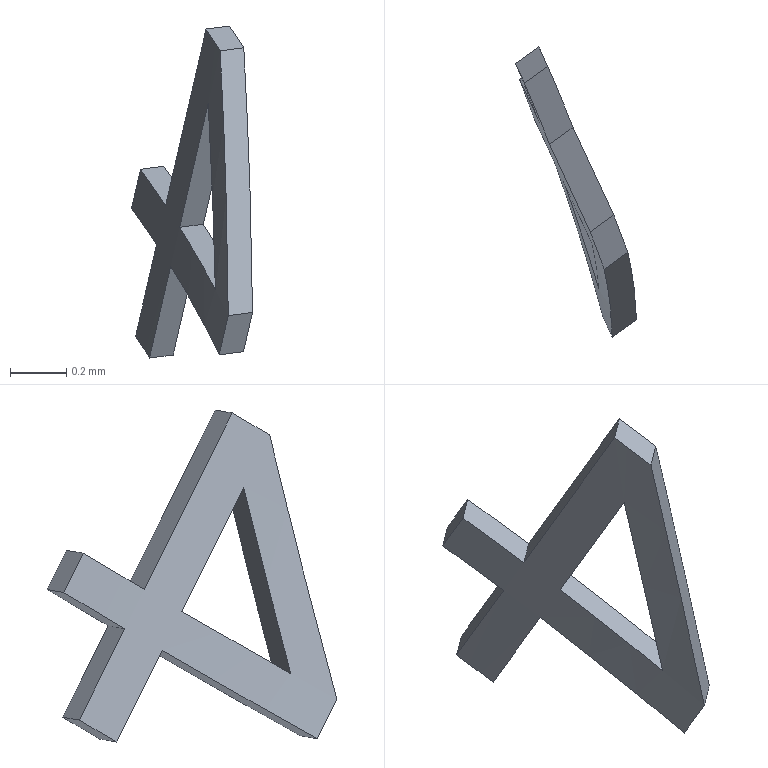Part | SolidWorks | features BaseBody 1 | 1 solid | 16 faces | box 0.4319 x 1.035 x 1.185 mm | volume 0.04699 mm3 | plane 14 | cylinder 2 | commonest cylinder face diameters 16.8 x1 17 x1
STEP:
#1=CARTESIAN_POINT('',(1974.754,-241.68,993.534));
#2=VERTEX_POINT('',#1);
#3=CARTESIAN_POINT('',(1974.725,-241.439,994.479));
#4=VERTEX_POINT('',#3);
#5=CARTESIAN_POINT('',(1974.754,-241.68,993.534));
#6=CARTESIAN_POINT('',(1974.752,-241.595,993.848));
#7=CARTESIAN_POINT('',(1974.742,-241.515,994.163));
#8=CARTESIAN_POINT('',(1974.725,-241.439,994.479));
#9=B_SPLINE_CURVE_WITH_KNOTS('',3,(#5,#6,#7,#8),.UNSPECIFIED.,.F.,.F.,(4,4),(0.,1.),.UNSPECIFIED.);
#10=EDGE_CURVE('',#2,#4,#9,.T.);
#11=ORIENTED_EDGE('',*,*,#10,.T.);
#12=CARTESIAN_POINT('',(1974.675,-241.306,994.556));
#13=VERTEX_POINT('',#12);
#14=CARTESIAN_POINT('',(1966.892,-244.458,994.777));
#15=DIRECTION('',(0.2015,-0.436,0.8771));
#16=DIRECTION('',(-0.7309,-0.6631,-0.1618));
#17=AXIS2_PLACEMENT_3D('',#14,#15,#16);
#18=CIRCLE('',#17,8.4);
#19=EDGE_CURVE('',#4,#13,#18,.T.);
#20=ORIENTED_EDGE('',*,*,#19,.T.);
#21=CARTESIAN_POINT('',(1974.53,-240.993,993.927));
#22=VERTEX_POINT('',#21);
#23=CARTESIAN_POINT('',(1975.233,-242.514,996.986));
#24=DIRECTION('',(-0.2015,0.436,-0.8771));
#25=VECTOR('',#24,1000.);
#26=LINE('',#23,#25);
#27=EDGE_CURVE('',#13,#22,#26,.T.);
#28=ORIENTED_EDGE('',*,*,#27,.T.);
#29=CARTESIAN_POINT('',(1974.441,-240.774,994.056));
#30=VERTEX_POINT('',#29);
#31=CARTESIAN_POINT('',(1966.747,-244.145,994.147));
#32=DIRECTION('',(0.2015,-0.436,0.8771));
#33=DIRECTION('',(-0.7309,-0.6631,-0.1618));
#34=AXIS2_PLACEMENT_3D('',#31,#32,#33);
#35=CIRCLE('',#34,8.4);
#36=EDGE_CURVE('',#22,#30,#35,.T.);
#37=ORIENTED_EDGE('',*,*,#36,.T.);
#38=CARTESIAN_POINT('',(1974.409,-240.705,993.916));
#39=VERTEX_POINT('',#38);
#40=CARTESIAN_POINT('',(1975.143,-242.295,997.115));
#41=DIRECTION('',(-0.2015,0.436,-0.8771));
#42=VECTOR('',#41,1000.);
#43=LINE('',#40,#42);
#44=EDGE_CURVE('',#30,#39,#43,.T.);
#45=ORIENTED_EDGE('',*,*,#44,.T.);
#46=CARTESIAN_POINT('',(1974.498,-240.923,993.787));
#47=VERTEX_POINT('',#46);
#48=CARTESIAN_POINT('',(1966.715,-244.076,994.007));
#49=DIRECTION('',(-0.2015,0.436,-0.8771));
#50=DIRECTION('',(-0.7309,-0.6631,-0.1618));
#51=AXIS2_PLACEMENT_3D('',#48,#49,#50);
#52=CIRCLE('',#51,8.4);
#53=EDGE_CURVE('',#39,#47,#52,.T.);
#54=ORIENTED_EDGE('',*,*,#53,.T.);
#55=CARTESIAN_POINT('',(1974.423,-240.761,993.46));
#56=VERTEX_POINT('',#55);
#57=CARTESIAN_POINT('',(1975.233,-242.514,996.986));
#58=DIRECTION('',(-0.2015,0.436,-0.8771));
#59=VECTOR('',#58,1000.);
#60=LINE('',#57,#59);
#61=EDGE_CURVE('',#47,#56,#60,.T.);
#62=ORIENTED_EDGE('',*,*,#61,.T.);
#63=CARTESIAN_POINT('',(1974.473,-240.894,993.382));
#64=VERTEX_POINT('',#63);
#65=CARTESIAN_POINT('',(1966.64,-243.913,993.681));
#66=DIRECTION('',(-0.2015,0.436,-0.8771));
#67=DIRECTION('',(-0.7309,-0.6631,-0.1618));
#68=AXIS2_PLACEMENT_3D('',#65,#66,#67);
#69=CIRCLE('',#68,8.4);
#70=EDGE_CURVE('',#56,#64,#69,.T.);
#71=ORIENTED_EDGE('',*,*,#70,.T.);
#72=CARTESIAN_POINT('',(1974.548,-241.057,993.709));
#73=VERTEX_POINT('',#72);
#74=CARTESIAN_POINT('',(1975.283,-242.647,996.908));
#75=DIRECTION('',(0.2015,-0.436,0.8771));
#76=VECTOR('',#75,1000.);
#77=LINE('',#74,#76);
#78=EDGE_CURVE('',#64,#73,#77,.T.);
#79=ORIENTED_EDGE('',*,*,#78,.T.);
#80=CARTESIAN_POINT('',(1974.722,-241.61,993.394));
#81=VERTEX_POINT('',#80);
#82=CARTESIAN_POINT('',(1966.715,-244.076,994.007));
#83=DIRECTION('',(-0.2015,0.436,-0.8771));
#84=DIRECTION('',(-0.7309,-0.6631,-0.1618));
#85=AXIS2_PLACEMENT_3D('',#82,#83,#84);
#86=CIRCLE('',#85,8.4);
#87=EDGE_CURVE('',#73,#81,#86,.T.);
#88=ORIENTED_EDGE('',*,*,#87,.T.);
#89=CARTESIAN_POINT('',(1975.457,-243.201,996.593));
#90=DIRECTION('',(-0.2015,0.436,-0.8771));
#91=VECTOR('',#90,1000.);
#92=LINE('',#89,#91);
#93=EDGE_CURVE('',#2,#81,#92,.T.);
#94=ORIENTED_EDGE('',*,*,#93,.F.);
#95=EDGE_LOOP('',(#11,#20,#28,#37,#45,#54,#62,#71,#79,#88,#94));
#96=FACE_OUTER_BOUND('',#95,.T.);
#97=CARTESIAN_POINT('',(1974.58,-241.126,993.849));
#98=VERTEX_POINT('',#97);
#99=CARTESIAN_POINT('',(1974.682,-241.347,994.292));
#100=VERTEX_POINT('',#99);
#101=CARTESIAN_POINT('',(1975.283,-242.647,996.908));
#102=DIRECTION('',(0.2015,-0.436,0.8771));
#103=VECTOR('',#102,1000.);
#104=LINE('',#101,#103);
#105=EDGE_CURVE('',#98,#100,#104,.T.);
#106=ORIENTED_EDGE('',*,*,#105,.T.);
#107=CARTESIAN_POINT('',(1974.708,-241.515,993.626));
#108=VERTEX_POINT('',#107);
#109=CARTESIAN_POINT('',(1974.708,-241.515,993.626));
#110=CARTESIAN_POINT('',(1974.703,-241.457,993.848));
#111=CARTESIAN_POINT('',(1974.694,-241.4,994.07));
#112=CARTESIAN_POINT('',(1974.682,-241.347,994.292));
#113=B_SPLINE_CURVE_WITH_KNOTS('',3,(#109,#110,#111,#112),.UNSPECIFIED.,.F.,.F.,(4,4),(0.,1.),.UNSPECIFIED.);
#114=EDGE_CURVE('',#108,#100,#113,.T.);
#115=ORIENTED_EDGE('',*,*,#114,.F.);
#116=CARTESIAN_POINT('',(1966.747,-244.145,994.147));
#117=DIRECTION('',(0.2015,-0.436,0.8771));
#118=DIRECTION('',(-0.7309,-0.6631,-0.1618));
#119=AXIS2_PLACEMENT_3D('',#116,#117,#118);
#120=CIRCLE('',#119,8.4);
#121=EDGE_CURVE('',#108,#98,#120,.T.);
#122=ORIENTED_EDGE('',*,*,#121,.T.);
#123=EDGE_LOOP('',(#106,#115,#122));
#124=FACE_BOUND('',#123,.T.);
#125=CARTESIAN_POINT('',(1967.45,-245.666,997.207));
#126=DIRECTION('',(0.2015,-0.436,0.8771));
#127=DIRECTION('',(-0.7309,-0.6631,-0.1618));
#128=AXIS2_PLACEMENT_3D('',#125,#126,#127);
#129=CYLINDRICAL_SURFACE('',#128,8.4);
#130=ADVANCED_FACE('',(#96,#124),#129,.F.);
#131=CARTESIAN_POINT('',(1974.84,-241.618,993.545));
#132=VERTEX_POINT('',#131);
#133=CARTESIAN_POINT('',(1974.808,-241.548,993.405));
#134=VERTEX_POINT('',#133);
#135=CARTESIAN_POINT('',(1974.824,-241.583,993.475));
#136=DIRECTION('',(-0.2015,0.436,-0.8771));
#137=VECTOR('',#136,1000.);
#138=LINE('',#135,#137);
#139=EDGE_CURVE('',#132,#134,#138,.T.);
#140=ORIENTED_EDGE('',*,*,#139,.F.);
#141=CARTESIAN_POINT('',(1974.797,-241.649,993.539));
#142=DIRECTION('',(-0.8088,-0.5792,-0.1022));
#143=VECTOR('',#142,1000.);
#144=LINE('',#141,#143);
#145=EDGE_CURVE('',#132,#2,#144,.T.);
#146=ORIENTED_EDGE('',*,*,#145,.T.);
#147=ORIENTED_EDGE('',*,*,#93,.T.);
#148=CARTESIAN_POINT('',(1974.765,-241.579,993.399));
#149=DIRECTION('',(-0.8088,-0.5792,-0.1022));
#150=VECTOR('',#149,1000.);
#151=LINE('',#148,#150);
#152=EDGE_CURVE('',#134,#81,#151,.T.);
#153=ORIENTED_EDGE('',*,*,#152,.F.);
#154=EDGE_LOOP('',(#140,#146,#147,#153));
#155=FACE_OUTER_BOUND('',#154,.T.);
#156=CARTESIAN_POINT('',(1980.21,-236.81,992.812));
#157=DIRECTION('',(-0.5526,0.6888,0.4693));
#158=DIRECTION('',(0.2015,-0.436,0.8771));
#159=AXIS2_PLACEMENT_3D('',#156,#157,#158);
#160=PLANE('',#159);
#161=ADVANCED_FACE('',(#155),#160,.F.);
#162=ORIENTED_EDGE('',*,*,#152,.T.);
#163=ORIENTED_EDGE('',*,*,#87,.F.);
#164=CARTESIAN_POINT('',(1974.632,-240.996,993.719));
#165=VERTEX_POINT('',#164);
#166=CARTESIAN_POINT('',(1974.59,-241.027,993.714));
#167=DIRECTION('',(-0.8088,-0.5792,-0.1022));
#168=VECTOR('',#167,1000.);
#169=LINE('',#166,#168);
#170=EDGE_CURVE('',#165,#73,#169,.T.);
#171=ORIENTED_EDGE('',*,*,#170,.F.);
#172=CARTESIAN_POINT('',(1966.715,-244.076,994.007));
#173=DIRECTION('',(-0.2015,0.436,-0.8771));
#174=DIRECTION('',(-0.7309,-0.6631,-0.1618));
#175=AXIS2_PLACEMENT_3D('',#172,#173,#174);
#176=CIRCLE('',#175,8.5);
#177=EDGE_CURVE('',#165,#134,#176,.T.);
#178=ORIENTED_EDGE('',*,*,#177,.T.);
#179=EDGE_LOOP('',(#162,#163,#171,#178));
#180=FACE_OUTER_BOUND('',#179,.T.);
#181=CARTESIAN_POINT('',(1980.167,-237.033,994.419));
#182=DIRECTION('',(-0.2015,0.436,-0.8771));
#183=DIRECTION('',(-0.5526,0.6888,0.4693));
#184=AXIS2_PLACEMENT_3D('',#181,#182,#183);
#185=PLANE('',#184);
#186=ADVANCED_FACE('',(#180),#185,.T.);
#187=ORIENTED_EDGE('',*,*,#170,.T.);
#188=ORIENTED_EDGE('',*,*,#78,.F.);
#189=CARTESIAN_POINT('',(1974.557,-240.834,993.393));
#190=VERTEX_POINT('',#189);
#191=CARTESIAN_POINT('',(1974.515,-240.864,993.388));
#192=DIRECTION('',(-0.8088,-0.5792,-0.1022));
#193=VECTOR('',#192,1000.);
#194=LINE('',#191,#193);
#195=EDGE_CURVE('',#190,#64,#194,.T.);
#196=ORIENTED_EDGE('',*,*,#195,.F.);
#197=CARTESIAN_POINT('',(1974.595,-240.915,993.556));
#198=DIRECTION('',(0.2015,-0.436,0.8771));
#199=VECTOR('',#198,1000.);
#200=LINE('',#197,#199);
#201=EDGE_CURVE('',#190,#165,#200,.T.);
#202=ORIENTED_EDGE('',*,*,#201,.T.);
#203=EDGE_LOOP('',(#187,#188,#196,#202));
#204=FACE_OUTER_BOUND('',#203,.T.);
#205=CARTESIAN_POINT('',(1980.091,-236.871,994.092));
#206=DIRECTION('',(0.5526,-0.6888,-0.4693));
#207=DIRECTION('',(-0.2015,0.436,-0.8771));
#208=AXIS2_PLACEMENT_3D('',#205,#206,#207);
#209=PLANE('',#208);
#210=ADVANCED_FACE('',(#204),#209,.T.);
#211=ORIENTED_EDGE('',*,*,#195,.T.);
#212=ORIENTED_EDGE('',*,*,#70,.F.);
#213=CARTESIAN_POINT('',(1974.507,-240.701,993.471));
#214=VERTEX_POINT('',#213);
#215=CARTESIAN_POINT('',(1974.465,-240.731,993.465));
#216=DIRECTION('',(-0.8088,-0.5792,-0.1022));
#217=VECTOR('',#216,1000.);
#218=LINE('',#215,#217);
#219=EDGE_CURVE('',#214,#56,#218,.T.);
#220=ORIENTED_EDGE('',*,*,#219,.F.);
#221=CARTESIAN_POINT('',(1966.64,-243.913,993.681));
#222=DIRECTION('',(-0.2015,0.436,-0.8771));
#223=DIRECTION('',(-0.7309,-0.6631,-0.1618));
#224=AXIS2_PLACEMENT_3D('',#221,#222,#223);
#225=CIRCLE('',#224,8.5);
#226=EDGE_CURVE('',#214,#190,#225,.T.);
#227=ORIENTED_EDGE('',*,*,#226,.T.);
#228=EDGE_LOOP('',(#211,#212,#220,#227));
#229=FACE_OUTER_BOUND('',#228,.T.);
#230=CARTESIAN_POINT('',(1982.308,-239.633,992.21));
#231=DIRECTION('',(-0.2015,0.436,-0.8771));
#232=DIRECTION('',(-0.5526,0.6888,0.4693));
#233=AXIS2_PLACEMENT_3D('',#230,#231,#232);
#234=PLANE('',#233);
#235=ADVANCED_FACE('',(#229),#234,.T.);
#236=ORIENTED_EDGE('',*,*,#219,.T.);
#237=ORIENTED_EDGE('',*,*,#61,.F.);
#238=CARTESIAN_POINT('',(1974.582,-240.863,993.797));
#239=VERTEX_POINT('',#238);
#240=CARTESIAN_POINT('',(1974.54,-240.893,993.792));
#241=DIRECTION('',(-0.8088,-0.5792,-0.1022));
#242=VECTOR('',#241,1000.);
#243=LINE('',#240,#242);
#244=EDGE_CURVE('',#239,#47,#243,.T.);
#245=ORIENTED_EDGE('',*,*,#244,.F.);
#246=CARTESIAN_POINT('',(1974.544,-240.782,993.634));
#247=DIRECTION('',(-0.2015,0.436,-0.8771));
#248=VECTOR('',#247,1000.);
#249=LINE('',#246,#248);
#250=EDGE_CURVE('',#239,#214,#249,.T.);
#251=ORIENTED_EDGE('',*,*,#250,.T.);
#252=EDGE_LOOP('',(#236,#237,#245,#251));
#253=FACE_OUTER_BOUND('',#252,.T.);
#254=CARTESIAN_POINT('',(1980.08,-236.925,994.492));
#255=DIRECTION('',(-0.5526,0.6888,0.4693));
#256=DIRECTION('',(0.2015,-0.436,0.8771));
#257=AXIS2_PLACEMENT_3D('',#254,#255,#256);
#258=PLANE('',#257);
#259=ADVANCED_FACE('',(#253),#258,.T.);
#260=ORIENTED_EDGE('',*,*,#244,.T.);
#261=ORIENTED_EDGE('',*,*,#53,.F.);
#262=CARTESIAN_POINT('',(1974.492,-240.645,993.926));
#263=VERTEX_POINT('',#262);
#264=CARTESIAN_POINT('',(1974.45,-240.675,993.921));
#265=DIRECTION('',(-0.8088,-0.5792,-0.1022));
#266=VECTOR('',#265,1000.);
#267=LINE('',#264,#266);
#268=EDGE_CURVE('',#263,#39,#267,.T.);
#269=ORIENTED_EDGE('',*,*,#268,.F.);
#270=CARTESIAN_POINT('',(1966.715,-244.076,994.007));
#271=DIRECTION('',(-0.2015,0.436,-0.8771));
#272=DIRECTION('',(-0.7309,-0.6631,-0.1618));
#273=AXIS2_PLACEMENT_3D('',#270,#271,#272);
#274=CIRCLE('',#273,8.5);
#275=EDGE_CURVE('',#263,#239,#274,.T.);
#276=ORIENTED_EDGE('',*,*,#275,.T.);
#277=EDGE_LOOP('',(#260,#261,#269,#276));
#278=FACE_OUTER_BOUND('',#277,.T.);
#279=CARTESIAN_POINT('',(1980.167,-237.033,994.419));
#280=DIRECTION('',(-0.2015,0.436,-0.8771));
#281=DIRECTION('',(-0.5526,0.6888,0.4693));
#282=AXIS2_PLACEMENT_3D('',#279,#280,#281);
#283=PLANE('',#282);
#284=ADVANCED_FACE('',(#278),#283,.T.);
#285=ORIENTED_EDGE('',*,*,#268,.T.);
#286=ORIENTED_EDGE('',*,*,#44,.F.);
#287=CARTESIAN_POINT('',(1974.524,-240.715,994.066));
#288=VERTEX_POINT('',#287);
#289=CARTESIAN_POINT('',(1974.482,-240.745,994.061));
#290=DIRECTION('',(-0.8088,-0.5792,-0.1022));
#291=VECTOR('',#290,1000.);
#292=LINE('',#289,#291);
#293=EDGE_CURVE('',#288,#30,#292,.T.);
#294=ORIENTED_EDGE('',*,*,#293,.F.);
#295=CARTESIAN_POINT('',(1974.508,-240.68,993.996));
#296=DIRECTION('',(-0.2015,0.436,-0.8771));
#297=VECTOR('',#296,1000.);
#298=LINE('',#295,#297);
#299=EDGE_CURVE('',#288,#263,#298,.T.);
#300=ORIENTED_EDGE('',*,*,#299,.T.);
#301=EDGE_LOOP('',(#285,#286,#294,#300));
#302=FACE_OUTER_BOUND('',#301,.T.);
#303=CARTESIAN_POINT('',(1979.968,-236.816,994.754));
#304=DIRECTION('',(-0.5526,0.6888,0.4693));
#305=DIRECTION('',(0.2015,-0.436,0.8771));
#306=AXIS2_PLACEMENT_3D('',#303,#304,#305);
#307=PLANE('',#306);
#308=ADVANCED_FACE('',(#302),#307,.T.);
#309=ORIENTED_EDGE('',*,*,#293,.T.);
#310=ORIENTED_EDGE('',*,*,#36,.F.);
#311=CARTESIAN_POINT('',(1974.614,-240.933,993.937));
#312=VERTEX_POINT('',#311);
#313=CARTESIAN_POINT('',(1974.572,-240.963,993.932));
#314=DIRECTION('',(-0.8088,-0.5792,-0.1022));
#315=VECTOR('',#314,1000.);
#316=LINE('',#313,#315);
#317=EDGE_CURVE('',#312,#22,#316,.T.);
#318=ORIENTED_EDGE('',*,*,#317,.F.);
#319=CARTESIAN_POINT('',(1966.747,-244.145,994.147));
#320=DIRECTION('',(0.2015,-0.436,0.8771));
#321=DIRECTION('',(-0.7309,-0.6631,-0.1618));
#322=AXIS2_PLACEMENT_3D('',#319,#320,#321);
#323=CIRCLE('',#322,8.5);
#324=EDGE_CURVE('',#312,#288,#323,.T.);
#325=ORIENTED_EDGE('',*,*,#324,.T.);
#326=EDGE_LOOP('',(#309,#310,#318,#325));
#327=FACE_OUTER_BOUND('',#326,.T.);
#328=CARTESIAN_POINT('',(1980.112,-236.995,994.632));
#329=DIRECTION('',(0.2015,-0.436,0.8771));
#330=DIRECTION('',(0.5526,-0.6888,-0.4693));
#331=AXIS2_PLACEMENT_3D('',#328,#329,#330);
#332=PLANE('',#331);
#333=ADVANCED_FACE('',(#327),#332,.T.);
#334=ORIENTED_EDGE('',*,*,#317,.T.);
#335=ORIENTED_EDGE('',*,*,#27,.F.);
#336=CARTESIAN_POINT('',(1974.759,-241.246,994.567));
#337=VERTEX_POINT('',#336);
#338=CARTESIAN_POINT('',(1974.717,-241.276,994.562));
#339=DIRECTION('',(-0.8088,-0.5792,-0.1022));
#340=VECTOR('',#339,1000.);
#341=LINE('',#338,#340);
#342=EDGE_CURVE('',#337,#13,#341,.T.);
#343=ORIENTED_EDGE('',*,*,#342,.F.);
#344=CARTESIAN_POINT('',(1974.686,-241.089,994.252));
#345=DIRECTION('',(-0.2015,0.436,-0.8771));
#346=VECTOR('',#345,1000.);
#347=LINE('',#344,#346);
#348=EDGE_CURVE('',#337,#312,#347,.T.);
#349=ORIENTED_EDGE('',*,*,#348,.T.);
#350=EDGE_LOOP('',(#334,#335,#343,#349));
#351=FACE_OUTER_BOUND('',#350,.T.);
#352=CARTESIAN_POINT('',(1980.08,-236.925,994.492));
#353=DIRECTION('',(-0.5526,0.6888,0.4693));
#354=DIRECTION('',(0.2015,-0.436,0.8771));
#355=AXIS2_PLACEMENT_3D('',#352,#353,#354);
#356=PLANE('',#355);
#357=ADVANCED_FACE('',(#351),#356,.T.);
#358=ORIENTED_EDGE('',*,*,#342,.T.);
#359=ORIENTED_EDGE('',*,*,#19,.F.);
#360=CARTESIAN_POINT('',(1974.809,-241.379,994.489));
#361=VERTEX_POINT('',#360);
#362=CARTESIAN_POINT('',(1974.767,-241.409,994.484));
#363=DIRECTION('',(-0.8088,-0.5792,-0.1022));
#364=VECTOR('',#363,1000.);
#365=LINE('',#362,#364);
#366=EDGE_CURVE('',#361,#4,#365,.T.);
#367=ORIENTED_EDGE('',*,*,#366,.F.);
#368=CARTESIAN_POINT('',(1966.892,-244.458,994.777));
#369=DIRECTION('',(0.2015,-0.436,0.8771));
#370=DIRECTION('',(-0.7309,-0.6631,-0.1618));
#371=AXIS2_PLACEMENT_3D('',#368,#369,#370);
#372=CIRCLE('',#371,8.5);
#373=EDGE_CURVE('',#361,#337,#372,.T.);
#374=ORIENTED_EDGE('',*,*,#373,.T.);
#375=EDGE_LOOP('',(#358,#359,#367,#374));
#376=FACE_OUTER_BOUND('',#375,.T.);
#377=CARTESIAN_POINT('',(1982.415,-239.999,993.428));
#378=DIRECTION('',(0.2015,-0.436,0.8771));
#379=DIRECTION('',(0.5526,-0.6888,-0.4693));
#380=AXIS2_PLACEMENT_3D('',#377,#378,#379);
#381=PLANE('',#380);
#382=ADVANCED_FACE('',(#376),#381,.T.);
#383=ORIENTED_EDGE('',*,*,#366,.T.);
#384=ORIENTED_EDGE('',*,*,#10,.F.);
#385=ORIENTED_EDGE('',*,*,#145,.F.);
#386=CARTESIAN_POINT('',(1974.84,-241.618,993.545));
#387=CARTESIAN_POINT('',(1974.839,-241.567,993.733));
#388=CARTESIAN_POINT('',(1974.835,-241.518,993.922));
#389=CARTESIAN_POINT('',(1974.828,-241.47,994.111));
#390=CARTESIAN_POINT('',(1974.82,-241.424,994.3));
#391=CARTESIAN_POINT('',(1974.809,-241.379,994.489));
#392=B_SPLINE_CURVE_WITH_KNOTS('',5,(#386,#387,#388,#389,#390,#391),.UNSPECIFIED.,.F.,.F.,(6,6),(0.,1.),.UNSPECIFIED.);
#393=EDGE_CURVE('',#132,#361,#392,.T.);
#394=ORIENTED_EDGE('',*,*,#393,.T.);
#395=EDGE_LOOP('',(#383,#384,#385,#394));
#396=FACE_OUTER_BOUND('',#395,.T.);
#397=CARTESIAN_POINT('',(1980.544,-237.533,994.265));
#398=DIRECTION('',(0.5491,-0.8058,0.2218));
#399=DIRECTION('',(0.2108,-0.1233,-0.9697));
#400=AXIS2_PLACEMENT_3D('',#397,#398,#399);
#401=PLANE('',#400);
#402=ADVANCED_FACE('',(#396),#401,.T.);
#403=CARTESIAN_POINT('',(1974.665,-241.066,993.859));
#404=VERTEX_POINT('',#403);
#405=CARTESIAN_POINT('',(1974.622,-241.096,993.854));
#406=DIRECTION('',(-0.8088,-0.5792,-0.1022));
#407=VECTOR('',#406,1000.);
#408=LINE('',#405,#407);
#409=EDGE_CURVE('',#404,#98,#408,.T.);
#410=ORIENTED_EDGE('',*,*,#409,.T.);
#411=ORIENTED_EDGE('',*,*,#121,.F.);
#412=CARTESIAN_POINT('',(1974.794,-241.454,993.637));
#413=VERTEX_POINT('',#412);
#414=CARTESIAN_POINT('',(1974.751,-241.484,993.632));
#415=DIRECTION('',(-0.8088,-0.5792,-0.1022));
#416=VECTOR('',#415,1000.);
#417=LINE('',#414,#416);
#418=EDGE_CURVE('',#413,#108,#417,.T.);
#419=ORIENTED_EDGE('',*,*,#418,.F.);
#420=CARTESIAN_POINT('',(1966.747,-244.145,994.147));
#421=DIRECTION('',(0.2015,-0.436,0.8771));
#422=DIRECTION('',(-0.7309,-0.6631,-0.1618));
#423=AXIS2_PLACEMENT_3D('',#420,#421,#422);
#424=CIRCLE('',#423,8.5);
#425=EDGE_CURVE('',#413,#404,#424,.T.);
#426=ORIENTED_EDGE('',*,*,#425,.T.);
#427=EDGE_LOOP('',(#410,#411,#419,#426));
#428=FACE_OUTER_BOUND('',#427,.T.);
#429=CARTESIAN_POINT('',(1980.112,-236.995,994.632));
#430=DIRECTION('',(0.2015,-0.436,0.8771));
#431=DIRECTION('',(0.5526,-0.6888,-0.4693));
#432=AXIS2_PLACEMENT_3D('',#429,#430,#431);
#433=PLANE('',#432);
#434=ADVANCED_FACE('',(#428),#433,.T.);
#435=CARTESIAN_POINT('',(1974.766,-241.286,994.303));
#436=VERTEX_POINT('',#435);
#437=CARTESIAN_POINT('',(1974.794,-241.454,993.637));
#438=CARTESIAN_POINT('',(1974.79,-241.419,993.77));
#439=CARTESIAN_POINT('',(1974.786,-241.385,993.903));
#440=CARTESIAN_POINT('',(1974.781,-241.351,994.036));
#441=CARTESIAN_POINT('',(1974.774,-241.318,994.169));
#442=CARTESIAN_POINT('',(1974.766,-241.286,994.303));
#443=B_SPLINE_CURVE_WITH_KNOTS('',5,(#437,#438,#439,#440,#441,#442),.UNSPECIFIED.,.F.,.F.,(6,6),(0.,1.),.UNSPECIFIED.);
#444=EDGE_CURVE('',#413,#436,#443,.T.);
#445=ORIENTED_EDGE('',*,*,#444,.F.);
#446=ORIENTED_EDGE('',*,*,#418,.T.);
#447=ORIENTED_EDGE('',*,*,#114,.T.);
#448=CARTESIAN_POINT('',(1974.724,-241.316,994.297));
#449=DIRECTION('',(-0.8088,-0.5792,-0.1022));
#450=VECTOR('',#449,1000.);
#451=LINE('',#448,#450);
#452=EDGE_CURVE('',#436,#100,#451,.T.);
#453=ORIENTED_EDGE('',*,*,#452,.F.);
#454=EDGE_LOOP('',(#445,#446,#447,#453));
#455=FACE_OUTER_BOUND('',#454,.T.);
#456=CARTESIAN_POINT('',(1980.443,-237.408,994.351));
#457=DIRECTION('',(0.5484,-0.8054,0.225));
#458=DIRECTION('',(0.2126,-0.1259,-0.969));
#459=AXIS2_PLACEMENT_3D('',#456,#457,#458);
#460=PLANE('',#459);
#461=ADVANCED_FACE('',(#455),#460,.F.);
#462=ORIENTED_EDGE('',*,*,#452,.T.);
#463=ORIENTED_EDGE('',*,*,#105,.F.);
#464=ORIENTED_EDGE('',*,*,#409,.F.);
#465=CARTESIAN_POINT('',(1974.716,-241.176,994.081));
#466=DIRECTION('',(0.2015,-0.436,0.8771));
#467=VECTOR('',#466,1000.);
#468=LINE('',#465,#467);
#469=EDGE_CURVE('',#404,#436,#468,.T.);
#470=ORIENTED_EDGE('',*,*,#469,.T.);
#471=EDGE_LOOP('',(#462,#463,#464,#470));
#472=FACE_OUTER_BOUND('',#471,.T.);
#473=CARTESIAN_POINT('',(1980.091,-236.871,994.092));
#474=DIRECTION('',(0.5526,-0.6888,-0.4693));
#475=DIRECTION('',(-0.2015,0.436,-0.8771));
#476=AXIS2_PLACEMENT_3D('',#473,#474,#475);
#477=PLANE('',#476);
#478=ADVANCED_FACE('',(#472),#477,.T.);
#479=ORIENTED_EDGE('',*,*,#139,.T.);
#480=ORIENTED_EDGE('',*,*,#177,.F.);
#481=ORIENTED_EDGE('',*,*,#201,.F.);
#482=ORIENTED_EDGE('',*,*,#226,.F.);
#483=ORIENTED_EDGE('',*,*,#250,.F.);
#484=ORIENTED_EDGE('',*,*,#275,.F.);
#485=ORIENTED_EDGE('',*,*,#299,.F.);
#486=ORIENTED_EDGE('',*,*,#324,.F.);
#487=ORIENTED_EDGE('',*,*,#348,.F.);
#488=ORIENTED_EDGE('',*,*,#373,.F.);
#489=ORIENTED_EDGE('',*,*,#393,.F.);
#490=EDGE_LOOP('',(#479,#480,#481,#482,#483,#484,#485,#486,#487,#488,#489));
#491=FACE_OUTER_BOUND('',#490,.T.);
#492=ORIENTED_EDGE('',*,*,#469,.F.);
#493=ORIENTED_EDGE('',*,*,#425,.F.);
#494=ORIENTED_EDGE('',*,*,#444,.T.);
#495=EDGE_LOOP('',(#492,#493,#494));
#496=FACE_BOUND('',#495,.T.);
#497=CARTESIAN_POINT('',(1967.45,-245.666,997.207));
#498=DIRECTION('',(0.2015,-0.436,0.8771));
#499=DIRECTION('',(-0.7309,-0.6631,-0.1618));
#500=AXIS2_PLACEMENT_3D('',#497,#498,#499);
#501=CYLINDRICAL_SURFACE('',#500,8.5);
#502=ADVANCED_FACE('',(#491,#496),#501,.T.);
#503=CLOSED_SHELL('',(#130,#161,#186,#210,#235,#259,#284,#308,#333,#357,#382,#402,#434,#461,#478,#502));
#504=MANIFOLD_SOLID_BREP('',#503);
#505=CARTESIAN_POINT('',(0.,0.,0.));
#506=DIRECTION('',(0.,0.,1.));
#507=DIRECTION('',(1.,0.,0.));
#508=AXIS2_PLACEMENT_3D('',#505,#506,#507);
#509=(LENGTH_UNIT()NAMED_UNIT(*)SI_UNIT(.MILLI.,.METRE.));
#510=UNCERTAINTY_MEASURE_WITH_UNIT(LENGTH_MEASURE(0.00001),#509,'','');
#511=(NAMED_UNIT(*)PLANE_ANGLE_UNIT()SI_UNIT($,.RADIAN.));
#512=(NAMED_UNIT(*)SI_UNIT($,.STERADIAN.)SOLID_ANGLE_UNIT());
#513=(GEOMETRIC_REPRESENTATION_CONTEXT(3)GLOBAL_UNCERTAINTY_ASSIGNED_CONTEXT((#510))GLOBAL_UNIT_ASSIGNED_CONTEXT((#509,#511,#512))REPRESENTATION_CONTEXT('',''));
#514=ADVANCED_BREP_SHAPE_REPRESENTATION('',(#504,#508),#513);